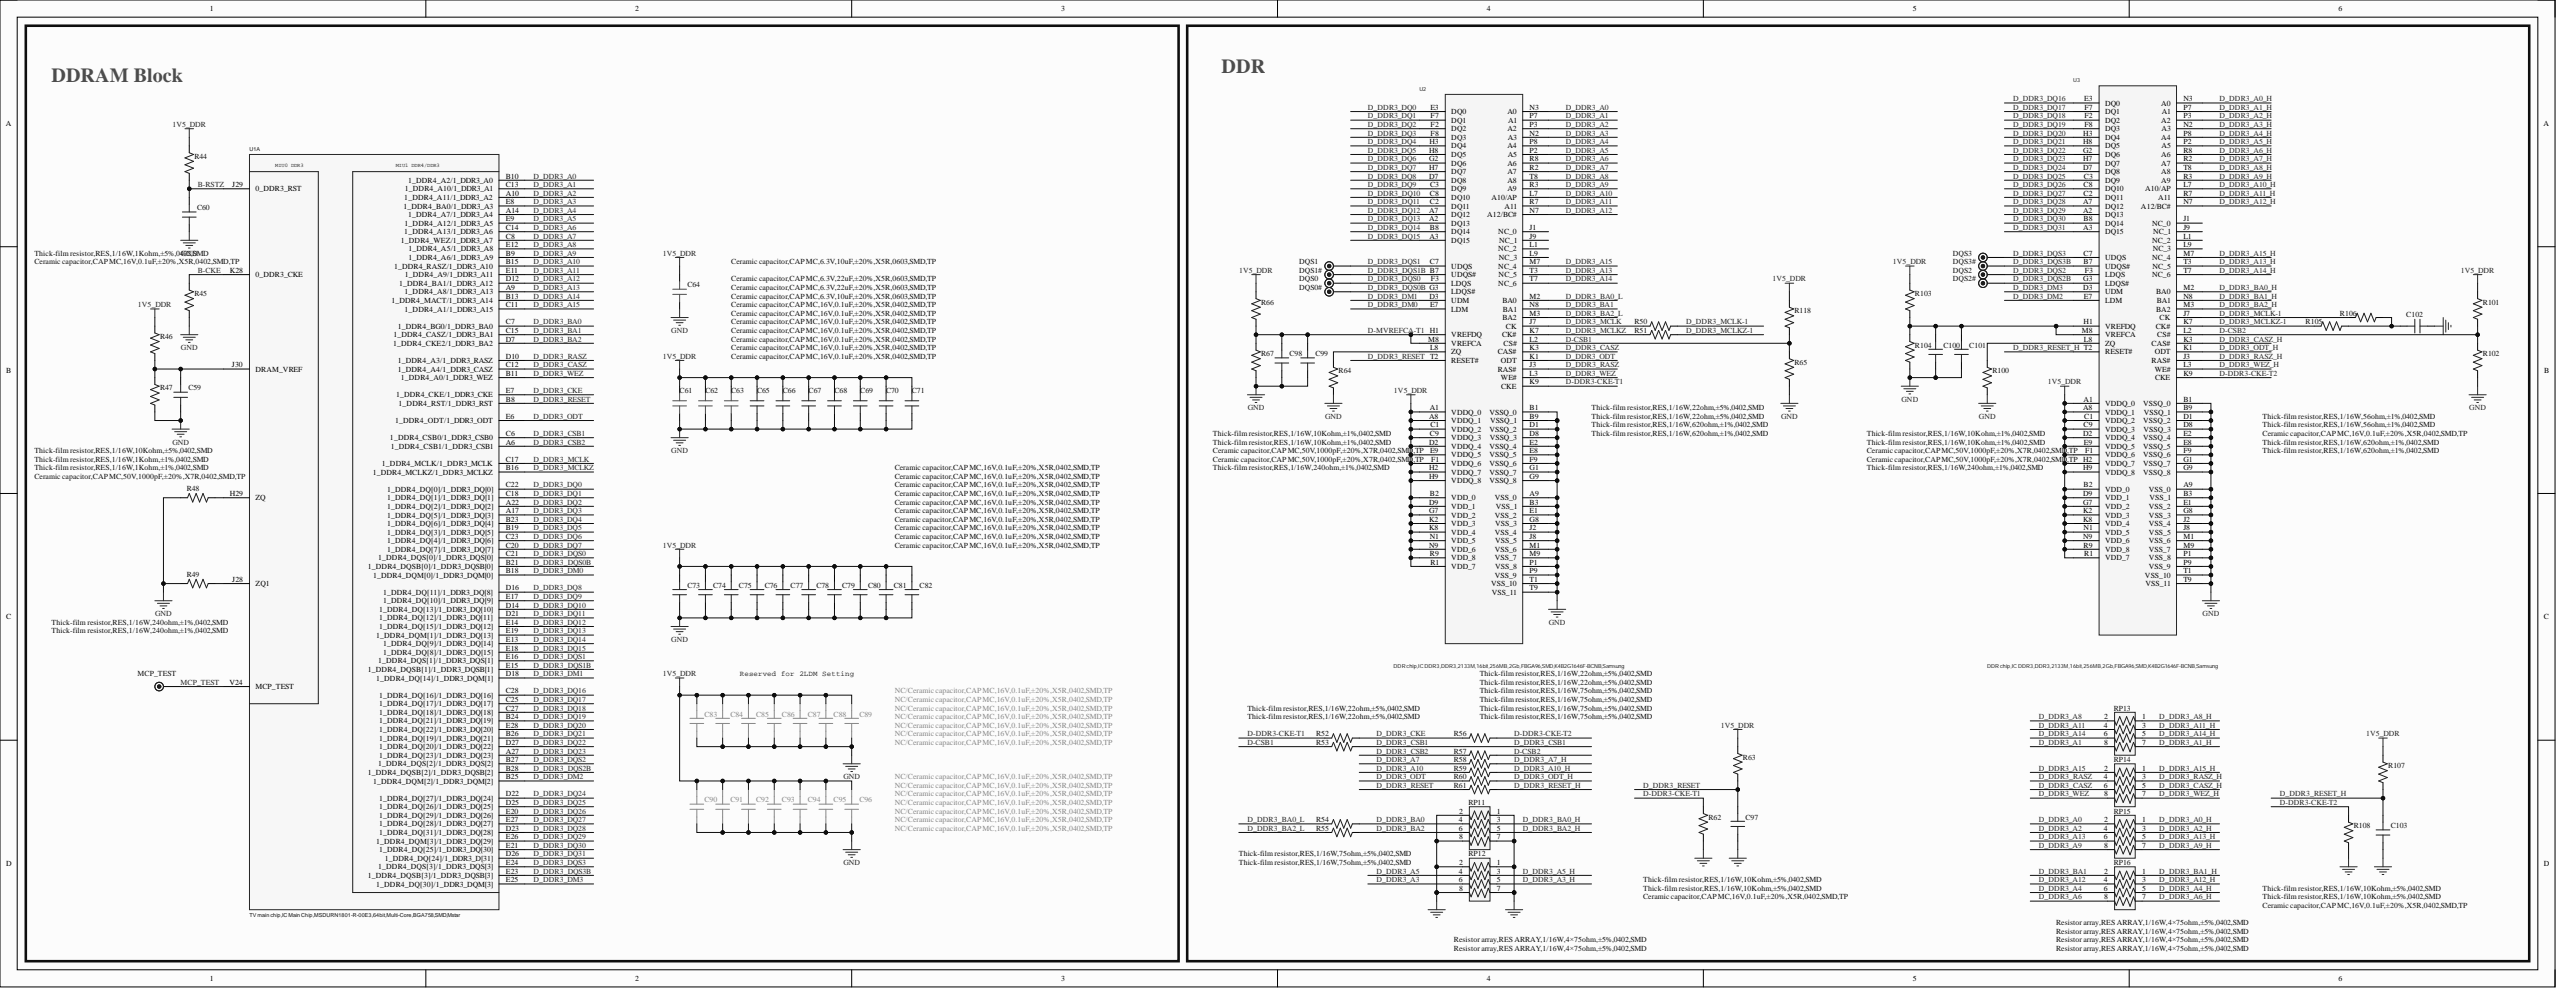Circuit board | Altium Designer | 1029 parts | 642 nets | one sheet of the schematic
Parts on this sheet (reference | value | footprint):
C59 | Ceramic capacitor,CAP MC,50V,1000pF,±20%,X7R,0402,SMD,TP | C0402
C60 | Ceramic capacitor,CAP MC,16V,0.1uF,±20%,X5R,0402,SMD,TP | C0402
C61 | Ceramic capacitor,CAP MC,6.3V,22uF,±20%,X5R,0603,SMD,TP | C0603
C62 | Ceramic capacitor,CAP MC,6.3V,22uF,±20%,X5R,0603,SMD,TP | C0603
C63 | Ceramic capacitor,CAP MC,6.3V,10uF,±20%,X5R,0603,SMD,TP | C0603
C64 | Ceramic capacitor,CAP MC,6.3V,10uF,±20%,X5R,0603,SMD,TP | C0603
C65 | Ceramic capacitor,CAP MC,16V,0.1uF,±20%,X5R,0402,SMD,TP | C0402
C66 | Ceramic capacitor,CAP MC,16V,0.1uF,±20%,X5R,0402,SMD,TP | C0402
C67 | Ceramic capacitor,CAP MC,16V,0.1uF,±20%,X5R,0402,SMD,TP | C0402
C68 | Ceramic capacitor,CAP MC,16V,0.1uF,±20%,X5R,0402,SMD,TP | C0402
C69 | Ceramic capacitor,CAP MC,16V,0.1uF,±20%,X5R,0402,SMD,TP | C0402
C70 | Ceramic capacitor,CAP MC,16V,0.1uF,±20%,X5R,0402,SMD,TP | C0402
C71 | Ceramic capacitor,CAP MC,16V,0.1uF,±20%,X5R,0402,SMD,TP | C0402
C73 | Ceramic capacitor,CAP MC,16V,0.1uF,±20%,X5R,0402,SMD,TP | C0402
C74 | Ceramic capacitor,CAP MC,16V,0.1uF,±20%,X5R,0402,SMD,TP | C0402
C75 | Ceramic capacitor,CAP MC,16V,0.1uF,±20%,X5R,0402,SMD,TP | C0402
C76 | Ceramic capacitor,CAP MC,16V,0.1uF,±20%,X5R,0402,SMD,TP | C0402
C77 | Ceramic capacitor,CAP MC,16V,0.1uF,±20%,X5R,0402,SMD,TP | C0402
C78 | Ceramic capacitor,CAP MC,16V,0.1uF,±20%,X5R,0402,SMD,TP | C0402
C79 | Ceramic capacitor,CAP MC,16V,0.1uF,±20%,X5R,0402,SMD,TP | C0402
C80 | Ceramic capacitor,CAP MC,16V,0.1uF,±20%,X5R,0402,SMD,TP | C0402
C81 | Ceramic capacitor,CAP MC,16V,0.1uF,±20%,X5R,0402,SMD,TP | C0402
C82 | Ceramic capacitor,CAP MC,16V,0.1uF,±20%,X5R,0402,SMD,TP | C0402
C83 | NC/Ceramic capacitor,CAP MC,16V,0.1uF,±20%,X5R,0402,SMD,TP | C0402
C84 | NC/Ceramic capacitor,CAP MC,16V,0.1uF,±20%,X5R,0402,SMD,TP | C0402
C85 | NC/Ceramic capacitor,CAP MC,16V,0.1uF,±20%,X5R,0402,SMD,TP | C0402
C86 | NC/Ceramic capacitor,CAP MC,16V,0.1uF,±20%,X5R,0402,SMD,TP | C0402
C88 | NC/Ceramic capacitor,CAP MC,16V,0.1uF,±20%,X5R,0402,SMD,TP | C0402
C89 | NC/Ceramic capacitor,CAP MC,16V,0.1uF,±20%,X5R,0402,SMD,TP | C0402
C90 | NC/Ceramic capacitor,CAP MC,16V,0.1uF,±20%,X5R,0402,SMD,TP | C0402
C91 | NC/Ceramic capacitor,CAP MC,16V,0.1uF,±20%,X5R,0402,SMD,TP | C0402
C92 | NC/Ceramic capacitor,CAP MC,16V,0.1uF,±20%,X5R,0402,SMD,TP | C0402
C93 | NC/Ceramic capacitor,CAP MC,16V,0.1uF,±20%,X5R,0402,SMD,TP | C0402
C95 | NC/Ceramic capacitor,CAP MC,16V,0.1uF,±20%,X5R,0402,SMD,TP | C0402
C96 | NC/Ceramic capacitor,CAP MC,16V,0.1uF,±20%,X5R,0402,SMD,TP | C0402
C97 | Ceramic capacitor,CAP MC,16V,0.1uF,±20%,X5R,0402,SMD,TP | C0402
C98 | Ceramic capacitor,CAP MC,50V,1000pF,±20%,X7R,0402,SMD,TP | C0402
C99 | Ceramic capacitor,CAP MC,50V,1000pF,±20%,X7R,0402,SMD,TP | C0402
C100 | Ceramic capacitor,CAP MC,50V,1000pF,±20%,X7R,0402,SMD,TP | C0402
C101 | Ceramic capacitor,CAP MC,50V,1000pF,±20%,X7R,0402,SMD,TP | C0402
C102 | Ceramic capacitor,CAP MC,16V,0.1uF,±20%,X5R,0402,SMD,TP | C0402
C103 | Ceramic capacitor,CAP MC,16V,0.1uF,±20%,X5R,0402,SMD,TP | C0402
DQS0 | TEST | TP-20
DQS0# | TEST | TP-20
DQS1 | TEST | TP-20
DQS1# | TEST | TP-20
DQS2 | TEST | TP-20
DQS2# | TEST | TP-20
DQS3 | TEST | TP-20
DQS3# | TEST | TP-20
MCP_TEST | TEST | TP-20
R44 | Thick-film resistor,RES,1/16W,1Kohm,±5%,0402,SMD | R0402
R45 | Thick-film resistor,RES,1/16W,10Kohm,±5%,0402,SMD | R0402
R46 | Thick-film resistor,RES,1/16W,1Kohm,±1%,0402,SMD | R0402
R47 | Thick-film resistor,RES,1/16W,1Kohm,±1%,0402,SMD | R0402
R48 | Thick-film resistor,RES,1/16W,240ohm,±1%,0402,SMD | R0402
R49 | Thick-film resistor,RES,1/16W,240ohm,±1%,0402,SMD | R0402
R50 | Thick-film resistor,RES,1/16W,22ohm,±5%,0402,SMD | R0402
R51 | Thick-film resistor,RES,1/16W,22ohm,±5%,0402,SMD | R0402
R52 | Thick-film resistor,RES,1/16W,22ohm,±5%,0402,SMD | R0402
R53 | Thick-film resistor,RES,1/16W,22ohm,±5%,0402,SMD | R0402
R54 | Thick-film resistor,RES,1/16W,75ohm,±5%,0402,SMD | R0402
R55 | Thick-film resistor,RES,1/16W,75ohm,±5%,0402,SMD | R0402
R56 | Thick-film resistor,RES,1/16W,22ohm,±5%,0402,SMD | R0402
R57 | Thick-film resistor,RES,1/16W,22ohm,±5%,0402,SMD | R0402
R58 | Thick-film resistor,RES,1/16W,75ohm,±5%,0402,SMD | R0402
R59 | Thick-film resistor,RES,1/16W,75ohm,±5%,0402,SMD | R0402
R60 | Thick-film resistor,RES,1/16W,75ohm,±5%,0402,SMD | R0402
R61 | Thick-film resistor,RES,1/16W,75ohm,±5%,0402,SMD | R0402
R62 | Thick-film resistor,RES,1/16W,10Kohm,±5%,0402,SMD | R0402
R63 | Thick-film resistor,RES,1/16W,10Kohm,±5%,0402,SMD | R0402
R64 | Thick-film resistor,RES,1/16W,240ohm,±1%,0402,SMD | R0402
R65 | Thick-film resistor,RES,1/16W,620ohm,±1%,0402,SMD | R0402
R66 | Thick-film resistor,RES,1/16W,10Kohm,±1%,0402,SMD | R0402
R67 | Thick-film resistor,RES,1/16W,10Kohm,±1%,0402,SMD | R0402
R100 | Thick-film resistor,RES,1/16W,240ohm,±1%,0402,SMD | R0402
R101 | Thick-film resistor,RES,1/16W,620ohm,±1%,0402,SMD | R0402
R102 | Thick-film resistor,RES,1/16W,620ohm,±1%,0402,SMD | R0402
R103 | Thick-film resistor,RES,1/16W,10Kohm,±1%,0402,SMD | R0402
R104 | Thick-film resistor,RES,1/16W,10Kohm,±1%,0402,SMD | R0402
R105 | Thick-film resistor,RES,1/16W,56ohm,±1%,0402,SMD | R0402
R106 | Thick-film resistor,RES,1/16W,56ohm,±1%,0402,SMD | R0402
R107 | Thick-film resistor,RES,1/16W,10Kohm,±5%,0402,SMD | R0402
R108 | Thick-film resistor,RES,1/16W,10Kohm,±5%,0402,SMD | R0402
R118 | Thick-film resistor,RES,1/16W,620ohm,±1%,0402,SMD | R0402
RP11 | Resistor array,RES ARRAY,1/16W,4×75ohm,±5%,0402,SMD | RA0402-MSD6886
RP12 | Resistor array,RES ARRAY,1/16W,4×75ohm,±5%,0402,SMD | RA0402-MSD6886
RP13 | Resistor array,RES ARRAY,1/16W,4×75ohm,±5%,0402,SMD | RA0402-MSD6886
RP14 | Resistor array,RES ARRAY,1/16W,4×75ohm,±5%,0402,SMD | RA0402-MSD6886
RP15 | Resistor array,RES ARRAY,1/16W,4×75ohm,±5%,0402,SMD | RA0402-MSD6886
RP16 | Resistor array,RES ARRAY,1/16W,4×75ohm,±5%,0402,SMD | RA0402-MSD6886
U1 | TV main chip,IC Main Chip,MSDURN1801-R-00E3,64bit,Multi-Core,BGA758,SMD,Mstar | BGA758/0.65
U2 | DDR chip,IC DDR3,DDR3,2133M,16bit,256MB,2Gb,FBGA96,SMD,K4B2G1646F-BCNB,Samsung | BGA96/0.8-1
U3 | DDR chip,IC DDR3,DDR3,2133M,16bit,256MB,2Gb,FBGA96,SMD,K4B2G1646F-BCNB,Samsung | BGA96/0.8-1
Nets of these parts (net: part-pin ...):
NetR100_2: R100-2 U3-L8
NetR64_2: R64-2 U2-L8
NetR49_2: R49-2 U1-J28
NetR48_2: R48-2 U1-H29
NetC102_2: C102-2 R105-1 R106-1
NetC100_2: C100-2 C101-2 R103-1 R104-2 U3-H1 U3-M8
NetC59_2: C59-2 R46-1 R47-2 U1-J30
MCP_TEST: MCP_TEST-1 U1-V24
GND: C59-1 C60-1 C61-1 C62-1 C63-1 C64-1 C65-1 C66-1 C67-1 C68-1 C69-1 C70-1 C71-1 C73-1 C74-1 C75-1 C76-1 C77-1 C78-1 C79-1 C80-1 C81-1 C82-1 C83-1 C84-1 C85-1 C86-1 C88-1 C89-1 C90-1 C91-1 C92-1 C93-1 C95-1 C96-1 C97-1 C98-1 C99-1 C100-1 C101-1 C102-1 C103-1 R45-1 R47-1 R48-1 R49-1 R62-1 R64-1 R65-1 R67-1 R100-1 R102-1 R104-1 R108-1 RP11-1 RP11-2 RP11-7 RP11-8 RP12-1 RP12-2 RP12-7 RP12-8 U1-A5 U1-C3 U1-C9 U1-D8 U1-D9 U1-F9 U1-G1 U1-G9 U1-H9 U1-J7 U1-J8 U1-J9 U1-K7 U1-K8 U1-L3 U1-L7 U1-L8 U1-L9 U1-M7 U1-N7 U1-N9 U1-P1 U1-R8 U1-R9 U1-T8 U1-T9 U2-A9 U2-B1 U2-B3 U2-B9 U2-D1 U2-D8 U2-E1 U2-E2 U2-E8 U2-F9 U2-G1 U2-G8 U2-G9 U2-J2 U2-J8 U2-M1 U2-M9 U2-P1 U2-P9 U2-T1 U2-T9 U3-A9 U3-B1 U3-B3 U3-B9 U3-D1 U3-D8 U3-E1 U3-E2 U3-E8 U3-F9 U3-G1 U3-G8 U3-G9 U3-J2 U3-J8 U3-M1 U3-M9 U3-P1 U3-P9 U3-T1 U3-T9
D_DDR3_WEZ_H: RP14-7 U3-L3
D_DDR3_WEZ: RP14-8 U1-B11 U2-L3
D_DDR3_RESET_H: C103-2 R61-2 R107-1 U3-T2
D_DDR3_RESET: C97-2 R61-1 R63-1 U1-B8 U2-T2
D_DDR3_RASZ_H: RP14-3 U3-J3
D_DDR3_RASZ: RP14-4 U1-D10 U2-J3
D_DDR3_ODT_H: R60-2 U3-K1
D_DDR3_ODT: R60-1 U1-E6 U2-K1
D_DDR3_MCLKZ-1: R51-2 R105-2 U3-K7
D_DDR3_MCLKZ: R51-1 U1-B16 U2-K7
D_DDR3_MCLK-1: R50-2 R106-2 U3-J7
D_DDR3_MCLK: R50-1 U1-C17 U2-J7
D_DDR3_DQS3B: DQS3#-1 U1-E23 U3-B7
D_DDR3_DQS3: DQS3-1 U1-E24 U3-C7
D_DDR3_DQS2B: DQS2#-1 U1-B28 U3-G3
D_DDR3_DQS2: DQS2-1 U1-B27 U3-F3
D_DDR3_DQS1B: DQS1#-1 U1-E15 U2-B7
D_DDR3_DQS1: DQS1-1 U1-E16 U2-C7
D_DDR3_DQS0B: DQS0#-1 U1-B21 U2-G3
D_DDR3_DQS0: DQS0-1 U1-C21 U2-F3
D_DDR3_DQ31: U1-D26 U3-A3
D_DDR3_DQ30: U1-E21 U3-B8
D_DDR3_DQ29: U1-E26 U3-A2
D_DDR3_DQ28: U1-D23 U3-A7
D_DDR3_DQ27: U1-E27 U3-C2
D_DDR3_DQ26: U1-E20 U3-C8
D_DDR3_DQ25: U1-D25 U3-C3
D_DDR3_DQ24: U1-D22 U3-D7
D_DDR3_DQ23: U1-A27 U3-H7
D_DDR3_DQ22: U1-D27 U3-G2
D_DDR3_DQ21: U1-B26 U3-H8
D_DDR3_DQ20: U1-E28 U3-H3
D_DDR3_DQ19: U1-B24 U3-F8
D_DDR3_DQ18: U1-C27 U3-F2
D_DDR3_DQ17: U1-C25 U3-F7
D_DDR3_DQ16: U1-C28 U3-E3
D_DDR3_DQ15: U1-E18 U2-A3
D_DDR3_DQ14: U1-E13 U2-B8
D_DDR3_DQ13: U1-E19 U2-A2
D_DDR3_DQ12: U1-E14 U2-A7
D_DDR3_DQ11: U1-D21 U2-C2
D_DDR3_DQ10: U1-D14 U2-C8
D_DDR3_DQ9: U1-E17 U2-C3
D_DDR3_DQ8: U1-D16 U2-D7
D_DDR3_DQ7: U1-C20 U2-H7
D_DDR3_DQ6: U1-C23 U2-G2
D_DDR3_DQ5: U1-B19 U2-H8
D_DDR3_DQ4: U1-B23 U2-H3
D_DDR3_DQ3: U1-A17 U2-F8
D_DDR3_DQ2: U1-A22 U2-F2
D_DDR3_DQ1: U1-C18 U2-F7
D_DDR3_DQ0: U1-C22 U2-E3
D_DDR3_DM3: U1-E25 U3-D3
D_DDR3_DM2: U1-B25 U3-E7
D_DDR3_DM1: U1-D18 U2-D3
D_DDR3_DM0: U1-B18 U2-E7
D_DDR3_CSB2: R57-1 U1-A6
D_DDR3_CSB1: R53-2 U1-C6
D_DDR3_CKE: R52-2 R56-1 U1-E7
D_DDR3_CASZ_H: RP14-5 U3-K3
D_DDR3_CASZ: RP14-6 U1-C12 U2-K3
D_DDR3_BA2_L: R55-1 U2-M3
D_DDR3_BA2_H: RP11-5 U3-M3
D_DDR3_BA2: R55-2 RP11-6 U1-D7
D_DDR3_BA1_H: RP16-1 U3-N8
D_DDR3_BA1: RP16-2 U1-C15 U2-N8
D_DDR3_BA0_L: R54-1 U2-M2
D_DDR3_BA0_H: RP11-3 U3-M2
D_DDR3_BA0: R54-2 RP11-4 U1-C7
D_DDR3_A15_H: RP14-1 U3-M7
D_DDR3_A15: RP14-2 U1-C11 U2-M7
D_DDR3_A14_H: RP13-5 U3-T7
D_DDR3_A14: RP13-6 U1-B13 U2-T7
D_DDR3_A13_H: RP15-5 U3-T3
D_DDR3_A13: RP15-6 U1-A9 U2-T3
D_DDR3_A12_H: RP16-3 U3-N7
D_DDR3_A12: RP16-4 U1-D12 U2-N7
D_DDR3_A11_H: RP13-3 U3-R7
D_DDR3_A11: RP13-4 U1-E11 U2-R7
D_DDR3_A10_H: R59-2 U3-L7
D_DDR3_A10: R59-1 U1-B15 U2-L7
D_DDR3_A9_H: RP15-7 U3-R3
D_DDR3_A9: RP15-8 U1-B9 U2-R3
D_DDR3_A8_H: RP13-1 U3-T8
D_DDR3_A8: RP13-2 U1-E12 U2-T8
D_DDR3_A7_H: R58-2 U3-R2
D_DDR3_A7: R58-1 U1-C8 U2-R2
D_DDR3_A6_H: RP16-7 U3-R8
D_DDR3_A6: RP16-8 U1-C14 U2-R8
D_DDR3_A5_H: RP12-3 U3-P2
D_DDR3_A5: RP12-4 U1-E9 U2-P2
D_DDR3_A4_H: RP16-5 U3-P8
D_DDR3_A4: RP16-6 U1-A14 U2-P8
D_DDR3_A3_H: RP12-5 U3-N2
D_DDR3_A3: RP12-6 U1-E8 U2-N2
D_DDR3_A2_H: RP15-3 U3-P3
D_DDR3_A2: RP15-4 U1-A10 U2-P3
D_DDR3_A1_H: RP13-7 U3-P7
D_DDR3_A1: RP13-8 U1-C13 U2-P7
D_DDR3_A0_H: RP15-1 U3-N3
D_DDR3_A0: RP15-2 U1-B10 U2-N3
D-MVREFCA-T1: C98-2 C99-2 R66-1 R67-2 U2-H1 U2-M8
D-DDR3-CKE-T2: R56-2 R108-2 U3-K9
D-DDR3-CKE-T1: R52-1 R62-2 U2-K9
D-CSB2: R57-2 R101-1 R102-2 U3-L2
D-CSB1: R53-1 R65-2 R118-1 U2-L2
B-RSTZ: C60-2 R44-1 U1-J29
B-CKE: R45-2 U1-K28
1V5_DDR: C61-2 C62-2 C63-2 C64-2 C65-2 C66-2 C67-2 C68-2 C69-2 C70-2 C71-2 C73-2 C74-2 C75-2 C76-2 C77-2 C78-2 C79-2 C80-2 C81-2 C82-2 C83-2 C84-2 C85-2 C86-2 C88-2 C89-2 C90-2 C91-2 C92-2 C93-2 C95-2 C96-2 R44-2 R46-2 R63-2 R66-2 R101-2 R103-2 R107-2 R118-2 U2-A1 U2-A8 U2-B2 U2-C1 U2-C9 U2-D2 U2-D9 U2-E9 U2-F1 U2-G7 U2-H2 U2-H9 U2-K2 U2-K8 U2-N1 U2-N9 U2-R1 U2-R9 U3-A1 U3-A8 U3-B2 U3-C1 U3-C9 U3-D2 U3-D9 U3-E9 U3-F1 U3-G7 U3-H2 U3-H9 U3-K2 U3-K8 U3-N1 U3-N9 U3-R1 U3-R9